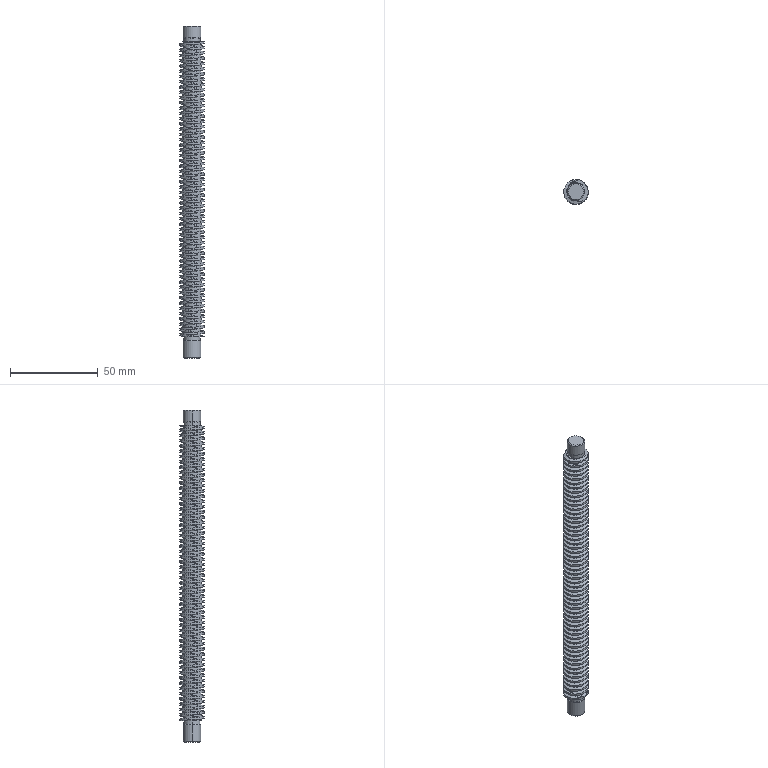Part | SolidWorks | features ICE 5, Chamfer 4, Extrusion 1, Helix 1, SweepCut 1 | 1 solid | 258 faces | box 14 x 14 x 189 mm | volume 21705 mm3 | cylinder 239 | cone 9 | plane 8 | spline 2 | commonest cylinder face diameters 10.5 x114 14 x114 9.5 x4 10 x4 4 x3